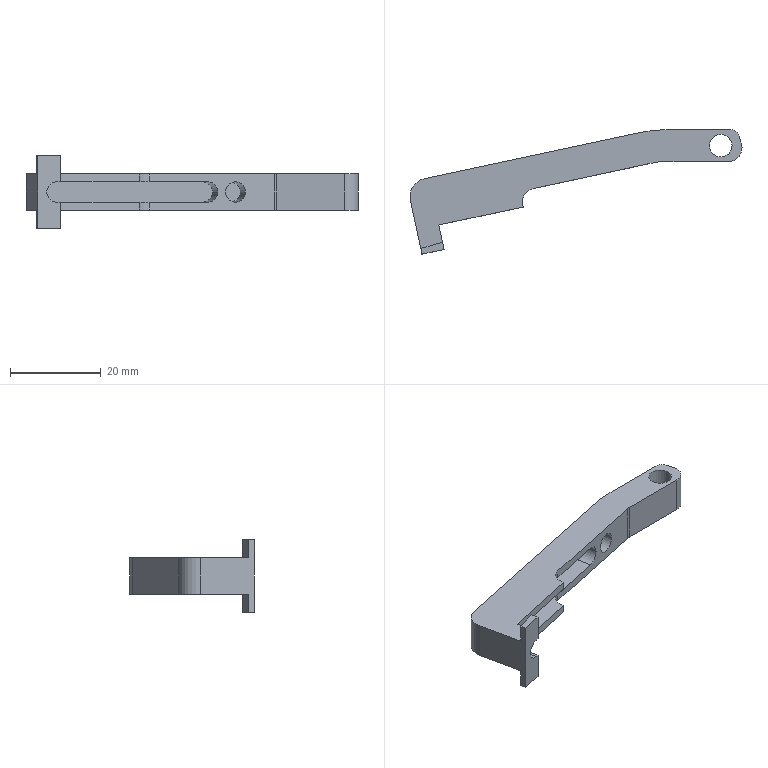Part | NX | features BREP 1 | 1 solid | 40 faces | box 73.222 x 27.429 x 16 mm | volume 3508 mm3 | plane 23 | cylinder 17 | commonest cylinder face diameters 6 x7 4.5 x5 5 x2 4 x1 8 x1 60 x1
STEP:
#1=CARTESIAN_POINT('',(-65.357,-7.291,4.));
#2=VERTEX_POINT('',#1);
#3=CARTESIAN_POINT('',(-68.43,-12.04,4.));
#4=VERTEX_POINT('',#3);
#5=CARTESIAN_POINT('',(-64.519,-11.202,4.));
#6=DIRECTION('',(0.,0.,1.));
#7=DIRECTION('',(1.,0.,0.));
#8=AXIS2_PLACEMENT_3D('',#5,#6,#7);
#9=CIRCLE('',#8,4.);
#10=EDGE_CURVE('',#2,#4,#9,.T.);
#11=ORIENTED_EDGE('',*,*,#10,.F.);
#12=CARTESIAN_POINT('',(-65.357,-7.291,-4.));
#13=VERTEX_POINT('',#12);
#14=CARTESIAN_POINT('',(-65.357,-7.291,4.));
#15=DIRECTION('',(0.,0.,1.));
#16=VECTOR('',#15,1000.);
#17=LINE('',#14,#16);
#18=EDGE_CURVE('',#13,#2,#17,.T.);
#19=ORIENTED_EDGE('',*,*,#18,.F.);
#20=CARTESIAN_POINT('',(-68.43,-12.04,-4.));
#21=VERTEX_POINT('',#20);
#22=CARTESIAN_POINT('',(-64.519,-11.202,-4.));
#23=DIRECTION('',(0.,0.,-1.));
#24=DIRECTION('',(1.,0.,0.));
#25=AXIS2_PLACEMENT_3D('',#22,#23,#24);
#26=CIRCLE('',#25,4.);
#27=EDGE_CURVE('',#21,#13,#26,.T.);
#28=ORIENTED_EDGE('',*,*,#27,.F.);
#29=CARTESIAN_POINT('',(-68.43,-12.04,-4.));
#30=DIRECTION('',(0.,0.,-1.));
#31=VECTOR('',#30,1000.);
#32=LINE('',#29,#31);
#33=EDGE_CURVE('',#4,#21,#32,.T.);
#34=ORIENTED_EDGE('',*,*,#33,.F.);
#35=EDGE_LOOP('',(#11,#19,#28,#34));
#36=FACE_BOUND('',#35,.T.);
#37=CARTESIAN_POINT('',(-64.519,-11.202,0.));
#38=DIRECTION('',(0.,0.,1.));
#39=DIRECTION('',(1.,0.,0.));
#40=AXIS2_PLACEMENT_3D('',#37,#38,#39);
#41=CYLINDRICAL_SURFACE('',#40,4.);
#42=ADVANCED_FACE('',(#36),#41,.T.);
#43=CARTESIAN_POINT('',(-66.144,-22.707,-8.));
#44=VERTEX_POINT('',#43);
#45=CARTESIAN_POINT('',(-61.334,-21.293,-8.));
#46=VERTEX_POINT('',#45);
#47=CARTESIAN_POINT('',(-56.523,-19.878,-8.));
#48=DIRECTION('',(0.9594,0.2821,0.));
#49=VECTOR('',#48,1000.);
#50=LINE('',#47,#49);
#51=EDGE_CURVE('',#44,#46,#50,.T.);
#52=ORIENTED_EDGE('',*,*,#51,.F.);
#53=CARTESIAN_POINT('',(-66.144,-22.707,-4.));
#54=VERTEX_POINT('',#53);
#55=CARTESIAN_POINT('',(-66.144,-22.707,0.));
#56=DIRECTION('',(0.,0.,-1.));
#57=VECTOR('',#56,1000.);
#58=LINE('',#55,#57);
#59=EDGE_CURVE('',#54,#44,#58,.T.);
#60=ORIENTED_EDGE('',*,*,#59,.F.);
#61=CARTESIAN_POINT('',(-61.334,-21.293,-4.));
#62=VERTEX_POINT('',#61);
#63=CARTESIAN_POINT('',(0.8821,-3.,-4.));
#64=DIRECTION('',(-0.9594,-0.2821,0.));
#65=VECTOR('',#64,1000.);
#66=LINE('',#63,#65);
#67=EDGE_CURVE('',#62,#54,#66,.T.);
#68=ORIENTED_EDGE('',*,*,#67,.F.);
#69=CARTESIAN_POINT('',(-61.334,-21.293,0.));
#70=DIRECTION('',(0.,0.,1.));
#71=VECTOR('',#70,1000.);
#72=LINE('',#69,#71);
#73=EDGE_CURVE('',#46,#62,#72,.T.);
#74=ORIENTED_EDGE('',*,*,#73,.F.);
#75=EDGE_LOOP('',(#52,#60,#68,#74));
#76=FACE_BOUND('',#75,.T.);
#77=CARTESIAN_POINT('',(-56.523,-19.878,0.));
#78=DIRECTION('',(0.2821,-0.9594,0.));
#79=DIRECTION('',(0.,0.,1.));
#80=AXIS2_PLACEMENT_3D('',#77,#78,#79);
#81=PLANE('',#80);
#82=ADVANCED_FACE('',(#76),#81,.F.);
#83=CARTESIAN_POINT('',(-66.144,-22.707,4.));
#84=VERTEX_POINT('',#83);
#85=CARTESIAN_POINT('',(-61.334,-21.293,4.));
#86=VERTEX_POINT('',#85);
#87=CARTESIAN_POINT('',(-56.523,-19.878,4.));
#88=DIRECTION('',(0.9594,0.2821,0.));
#89=VECTOR('',#88,1000.);
#90=LINE('',#87,#89);
#91=EDGE_CURVE('',#84,#86,#90,.T.);
#92=ORIENTED_EDGE('',*,*,#91,.F.);
#93=CARTESIAN_POINT('',(-66.144,-22.707,8.));
#94=VERTEX_POINT('',#93);
#95=CARTESIAN_POINT('',(-66.144,-22.707,0.));
#96=DIRECTION('',(0.,0.,-1.));
#97=VECTOR('',#96,1000.);
#98=LINE('',#95,#97);
#99=EDGE_CURVE('',#94,#84,#98,.T.);
#100=ORIENTED_EDGE('',*,*,#99,.F.);
#101=CARTESIAN_POINT('',(-61.334,-21.293,8.));
#102=VERTEX_POINT('',#101);
#103=CARTESIAN_POINT('',(-56.523,-19.878,8.));
#104=DIRECTION('',(-0.9594,-0.2821,0.));
#105=VECTOR('',#104,1000.);
#106=LINE('',#103,#105);
#107=EDGE_CURVE('',#102,#94,#106,.T.);
#108=ORIENTED_EDGE('',*,*,#107,.F.);
#109=CARTESIAN_POINT('',(-61.334,-21.293,0.));
#110=DIRECTION('',(0.,0.,1.));
#111=VECTOR('',#110,1000.);
#112=LINE('',#109,#111);
#113=EDGE_CURVE('',#86,#102,#112,.T.);
#114=ORIENTED_EDGE('',*,*,#113,.F.);
#115=EDGE_LOOP('',(#92,#100,#108,#114));
#116=FACE_BOUND('',#115,.T.);
#117=CARTESIAN_POINT('',(-56.523,-19.878,0.));
#118=DIRECTION('',(0.2821,-0.9594,0.));
#119=DIRECTION('',(0.,0.,1.));
#120=AXIS2_PLACEMENT_3D('',#117,#118,#119);
#121=PLANE('',#120);
#122=ADVANCED_FACE('',(#116),#121,.F.);
#123=CARTESIAN_POINT('',(-60.993,-22.881,2.25));
#124=VERTEX_POINT('',#123);
#125=CARTESIAN_POINT('',(-60.993,-22.881,8.));
#126=VERTEX_POINT('',#125);
#127=CARTESIAN_POINT('',(-60.993,-22.881,2.25));
#128=DIRECTION('',(0.,0.,1.));
#129=VECTOR('',#128,1000.);
#130=LINE('',#127,#129);
#131=EDGE_CURVE('',#124,#126,#130,.T.);
#132=ORIENTED_EDGE('',*,*,#131,.T.);
#133=CARTESIAN_POINT('',(-65.882,-23.929,8.));
#134=VERTEX_POINT('',#133);
#135=CARTESIAN_POINT('',(-65.882,-23.929,8.));
#136=DIRECTION('',(-0.9778,-0.2095,0.));
#137=VECTOR('',#136,1000.);
#138=LINE('',#135,#137);
#139=EDGE_CURVE('',#126,#134,#138,.T.);
#140=ORIENTED_EDGE('',*,*,#139,.T.);
#141=CARTESIAN_POINT('',(-65.882,-23.929,-8.));
#142=VERTEX_POINT('',#141);
#143=CARTESIAN_POINT('',(-65.882,-23.929,-8.));
#144=DIRECTION('',(0.,0.,-1.));
#145=VECTOR('',#144,1000.);
#146=LINE('',#143,#145);
#147=EDGE_CURVE('',#134,#142,#146,.T.);
#148=ORIENTED_EDGE('',*,*,#147,.T.);
#149=CARTESIAN_POINT('',(-60.993,-22.881,-8.));
#150=VERTEX_POINT('',#149);
#151=CARTESIAN_POINT('',(-65.882,-23.929,-8.));
#152=DIRECTION('',(0.9778,0.2095,0.));
#153=VECTOR('',#152,1000.);
#154=LINE('',#151,#153);
#155=EDGE_CURVE('',#142,#150,#154,.T.);
#156=ORIENTED_EDGE('',*,*,#155,.T.);
#157=CARTESIAN_POINT('',(-60.993,-22.881,-2.25));
#158=VERTEX_POINT('',#157);
#159=CARTESIAN_POINT('',(-60.993,-22.881,-8.));
#160=DIRECTION('',(0.,0.,1.));
#161=VECTOR('',#160,1000.);
#162=LINE('',#159,#161);
#163=EDGE_CURVE('',#150,#158,#162,.T.);
#164=ORIENTED_EDGE('',*,*,#163,.T.);
#165=CARTESIAN_POINT('',(-61.727,-23.039,-2.25));
#166=VERTEX_POINT('',#165);
#167=CARTESIAN_POINT('',(-61.727,-23.039,-2.25));
#168=DIRECTION('',(-0.9778,-0.2095,0.));
#169=VECTOR('',#168,1000.);
#170=LINE('',#167,#169);
#171=EDGE_CURVE('',#158,#166,#170,.T.);
#172=ORIENTED_EDGE('',*,*,#171,.T.);
#173=CARTESIAN_POINT('',(-61.727,-23.039,2.25));
#174=VERTEX_POINT('',#173);
#175=CARTESIAN_POINT('',(-61.727,-23.039,0.));
#176=DIRECTION('',(-0.2095,0.9778,0.));
#177=DIRECTION('',(0.9778,0.2095,0.));
#178=AXIS2_PLACEMENT_3D('',#175,#176,#177);
#179=CIRCLE('',#178,2.25);
#180=EDGE_CURVE('',#166,#174,#179,.T.);
#181=ORIENTED_EDGE('',*,*,#180,.T.);
#182=CARTESIAN_POINT('',(-60.993,-22.881,2.25));
#183=DIRECTION('',(0.9778,0.2095,0.));
#184=VECTOR('',#183,1000.);
#185=LINE('',#182,#184);
#186=EDGE_CURVE('',#174,#124,#185,.T.);
#187=ORIENTED_EDGE('',*,*,#186,.T.);
#188=EDGE_LOOP('',(#132,#140,#148,#156,#164,#172,#181,#187));
#189=FACE_BOUND('',#188,.T.);
#190=CARTESIAN_POINT('',(-61.727,-23.039,0.));
#191=DIRECTION('',(0.2095,-0.9778,0.));
#192=DIRECTION('',(0.9778,0.2095,0.));
#193=AXIS2_PLACEMENT_3D('',#190,#191,#192);
#194=PLANE('',#193);
#195=ADVANCED_FACE('',(#189),#194,.T.);
#196=ORIENTED_EDGE('',*,*,#73,.T.);
#197=CARTESIAN_POINT('',(-62.146,-17.504,-4.));
#198=VERTEX_POINT('',#197);
#199=CARTESIAN_POINT('',(-61.412,-20.926,-4.));
#200=DIRECTION('',(-0.2095,0.9778,0.));
#201=VECTOR('',#200,1000.);
#202=LINE('',#199,#201);
#203=EDGE_CURVE('',#62,#198,#202,.T.);
#204=ORIENTED_EDGE('',*,*,#203,.T.);
#205=CARTESIAN_POINT('',(-62.146,-17.504,-2.25));
#206=VERTEX_POINT('',#205);
#207=CARTESIAN_POINT('',(-62.146,-17.504,-8.));
#208=DIRECTION('',(0.,0.,1.));
#209=VECTOR('',#208,1000.);
#210=LINE('',#207,#209);
#211=EDGE_CURVE('',#198,#206,#210,.T.);
#212=ORIENTED_EDGE('',*,*,#211,.T.);
#213=CARTESIAN_POINT('',(-60.993,-22.881,-2.25));
#214=DIRECTION('',(-0.2095,0.9778,0.));
#215=VECTOR('',#214,1000.);
#216=LINE('',#213,#215);
#217=EDGE_CURVE('',#158,#206,#216,.T.);
#218=ORIENTED_EDGE('',*,*,#217,.F.);
#219=ORIENTED_EDGE('',*,*,#163,.F.);
#220=CARTESIAN_POINT('',(-60.993,-22.881,-8.));
#221=DIRECTION('',(-0.2095,0.9778,0.));
#222=VECTOR('',#221,1000.);
#223=LINE('',#220,#222);
#224=EDGE_CURVE('',#150,#46,#223,.T.);
#225=ORIENTED_EDGE('',*,*,#224,.T.);
#226=EDGE_LOOP('',(#196,#204,#212,#218,#219,#225));
#227=FACE_BOUND('',#226,.T.);
#228=CARTESIAN_POINT('',(-60.993,-22.881,-8.));
#229=DIRECTION('',(-0.9778,-0.2095,0.));
#230=DIRECTION('',(0.2095,-0.9778,0.));
#231=AXIS2_PLACEMENT_3D('',#228,#229,#230);
#232=PLANE('',#231);
#233=ADVANCED_FACE('',(#227),#232,.F.);
#234=CARTESIAN_POINT('',(-62.146,-17.504,4.));
#235=VERTEX_POINT('',#234);
#236=CARTESIAN_POINT('',(-61.412,-20.926,4.));
#237=DIRECTION('',(-0.2095,0.9778,0.));
#238=VECTOR('',#237,1000.);
#239=LINE('',#236,#238);
#240=EDGE_CURVE('',#86,#235,#239,.T.);
#241=ORIENTED_EDGE('',*,*,#240,.F.);
#242=ORIENTED_EDGE('',*,*,#113,.T.);
#243=CARTESIAN_POINT('',(-60.993,-22.881,8.));
#244=DIRECTION('',(-0.2095,0.9778,0.));
#245=VECTOR('',#244,1000.);
#246=LINE('',#243,#245);
#247=EDGE_CURVE('',#126,#102,#246,.T.);
#248=ORIENTED_EDGE('',*,*,#247,.F.);
#249=ORIENTED_EDGE('',*,*,#131,.F.);
#250=CARTESIAN_POINT('',(-62.146,-17.504,2.25));
#251=VERTEX_POINT('',#250);
#252=CARTESIAN_POINT('',(-60.993,-22.881,2.25));
#253=DIRECTION('',(-0.2095,0.9778,0.));
#254=VECTOR('',#253,1000.);
#255=LINE('',#252,#254);
#256=EDGE_CURVE('',#124,#251,#255,.T.);
#257=ORIENTED_EDGE('',*,*,#256,.T.);
#258=CARTESIAN_POINT('',(-62.146,-17.504,2.25));
#259=DIRECTION('',(0.,0.,1.));
#260=VECTOR('',#259,1000.);
#261=LINE('',#258,#260);
#262=EDGE_CURVE('',#251,#235,#261,.T.);
#263=ORIENTED_EDGE('',*,*,#262,.T.);
#264=EDGE_LOOP('',(#241,#242,#248,#249,#257,#263));
#265=FACE_BOUND('',#264,.T.);
#266=CARTESIAN_POINT('',(-60.993,-22.881,2.25));
#267=DIRECTION('',(-0.9778,-0.2095,0.));
#268=DIRECTION('',(0.2095,-0.9778,0.));
#269=AXIS2_PLACEMENT_3D('',#266,#267,#268);
#270=PLANE('',#269);
#271=ADVANCED_FACE('',(#265),#270,.F.);
#272=CARTESIAN_POINT('',(-64.765,-8.86,2.25));
#273=VERTEX_POINT('',#272);
#274=CARTESIAN_POINT('',(-73.303,30.984,2.25));
#275=DIRECTION('',(0.2095,-0.9778,0.));
#276=VECTOR('',#275,1000.);
#277=LINE('',#274,#276);
#278=EDGE_CURVE('',#273,#174,#277,.T.);
#279=ORIENTED_EDGE('',*,*,#278,.T.);
#280=ORIENTED_EDGE('',*,*,#180,.F.);
#281=CARTESIAN_POINT('',(-64.765,-8.86,-2.25));
#282=VERTEX_POINT('',#281);
#283=CARTESIAN_POINT('',(-73.303,30.984,-2.25));
#284=DIRECTION('',(0.2095,-0.9778,0.));
#285=VECTOR('',#284,1000.);
#286=LINE('',#283,#285);
#287=EDGE_CURVE('',#282,#166,#286,.T.);
#288=ORIENTED_EDGE('',*,*,#287,.F.);
#289=CARTESIAN_POINT('',(-64.765,-8.86,0.));
#290=DIRECTION('',(0.2095,-0.9778,0.));
#291=DIRECTION('',(-0.9778,-0.2095,0.));
#292=AXIS2_PLACEMENT_3D('',#289,#290,#291);
#293=CIRCLE('',#292,2.25);
#294=EDGE_CURVE('',#273,#282,#293,.T.);
#295=ORIENTED_EDGE('',*,*,#294,.F.);
#296=EDGE_LOOP('',(#279,#280,#288,#295));
#297=FACE_BOUND('',#296,.T.);
#298=CARTESIAN_POINT('',(-73.303,30.984,0.));
#299=DIRECTION('',(0.2095,-0.9778,0.));
#300=DIRECTION('',(0.9778,0.2095,0.));
#301=AXIS2_PLACEMENT_3D('',#298,#299,#300);
#302=CYLINDRICAL_SURFACE('',#301,2.25);
#303=ADVANCED_FACE('',(#297),#302,.F.);
#304=ORIENTED_EDGE('',*,*,#294,.T.);
#305=CARTESIAN_POINT('',(-29.564,-1.317,-2.25));
#306=VERTEX_POINT('',#305);
#307=CARTESIAN_POINT('',(-64.765,-8.86,-2.25));
#308=DIRECTION('',(0.9778,0.2095,0.));
#309=VECTOR('',#308,1000.);
#310=LINE('',#307,#309);
#311=EDGE_CURVE('',#282,#306,#310,.T.);
#312=ORIENTED_EDGE('',*,*,#311,.T.);
#313=CARTESIAN_POINT('',(-27.364,-0.846,0.));
#314=VERTEX_POINT('',#313);
#315=CARTESIAN_POINT('',(-29.564,-1.317,0.));
#316=DIRECTION('',(0.2095,-0.9778,0.));
#317=DIRECTION('',(-0.9778,-0.2095,0.));
#318=AXIS2_PLACEMENT_3D('',#315,#316,#317);
#319=CIRCLE('',#318,2.25);
#320=EDGE_CURVE('',#306,#314,#319,.T.);
#321=ORIENTED_EDGE('',*,*,#320,.T.);
#322=CARTESIAN_POINT('',(-29.564,-1.317,2.25));
#323=VERTEX_POINT('',#322);
#324=CARTESIAN_POINT('',(-29.564,-1.317,0.));
#325=DIRECTION('',(0.2095,-0.9778,0.));
#326=DIRECTION('',(-0.9778,-0.2095,0.));
#327=AXIS2_PLACEMENT_3D('',#324,#325,#326);
#328=CIRCLE('',#327,2.25);
#329=EDGE_CURVE('',#314,#323,#328,.T.);
#330=ORIENTED_EDGE('',*,*,#329,.T.);
#331=CARTESIAN_POINT('',(-64.765,-8.86,2.25));
#332=DIRECTION('',(-0.9778,-0.2095,0.));
#333=VECTOR('',#332,1000.);
#334=LINE('',#331,#333);
#335=EDGE_CURVE('',#323,#273,#334,.T.);
#336=ORIENTED_EDGE('',*,*,#335,.T.);
#337=EDGE_LOOP('',(#304,#312,#321,#330,#336));
#338=FACE_BOUND('',#337,.T.);
#339=CARTESIAN_POINT('',(-23.453,-0.007849,0.));
#340=DIRECTION('',(-0.2095,0.9778,0.));
#341=DIRECTION('',(-0.9778,-0.2095,0.));
#342=AXIS2_PLACEMENT_3D('',#339,#340,#341);
#343=PLANE('',#342);
#344=ADVANCED_FACE('',(#338),#343,.F.);
#345=CARTESIAN_POINT('',(-43.672,-13.034,2.25));
#346=VERTEX_POINT('',#345);
#347=CARTESIAN_POINT('',(-43.739,-12.405,2.25));
#348=VERTEX_POINT('',#347);
#349=CARTESIAN_POINT('',(-40.739,-12.405,2.25));
#350=DIRECTION('',(0.,0.,-1.));
#351=DIRECTION('',(1.,0.,0.));
#352=AXIS2_PLACEMENT_3D('',#349,#350,#351);
#353=CIRCLE('',#352,3.);
#354=EDGE_CURVE('',#346,#348,#353,.T.);
#355=ORIENTED_EDGE('',*,*,#354,.F.);
#356=CARTESIAN_POINT('',(-43.567,-13.522,2.25));
#357=VERTEX_POINT('',#356);
#358=CARTESIAN_POINT('',(-43.567,-13.522,2.25));
#359=DIRECTION('',(-0.2095,0.9778,0.));
#360=VECTOR('',#359,1000.);
#361=LINE('',#358,#360);
#362=EDGE_CURVE('',#357,#346,#361,.T.);
#363=ORIENTED_EDGE('',*,*,#362,.F.);
#364=CARTESIAN_POINT('',(-62.879,-17.661,2.25));
#365=DIRECTION('',(-0.9778,-0.2095,0.));
#366=VECTOR('',#365,1000.);
#367=LINE('',#364,#366);
#368=EDGE_CURVE('',#357,#251,#367,.T.);
#369=ORIENTED_EDGE('',*,*,#368,.T.);
#370=ORIENTED_EDGE('',*,*,#256,.F.);
#371=ORIENTED_EDGE('',*,*,#186,.F.);
#372=ORIENTED_EDGE('',*,*,#278,.F.);
#373=ORIENTED_EDGE('',*,*,#335,.F.);
#374=CARTESIAN_POINT('',(-28.411,-6.695,2.25));
#375=VERTEX_POINT('',#374);
#376=CARTESIAN_POINT('',(-38.102,38.527,2.25));
#377=DIRECTION('',(0.2095,-0.9778,0.));
#378=VECTOR('',#377,1000.);
#379=LINE('',#376,#378);
#380=EDGE_CURVE('',#323,#375,#379,.T.);
#381=ORIENTED_EDGE('',*,*,#380,.T.);
#382=CARTESIAN_POINT('',(-41.367,-9.472,2.25));
#383=VERTEX_POINT('',#382);
#384=CARTESIAN_POINT('',(-67.768,-15.129,2.25));
#385=DIRECTION('',(0.9778,0.2095,0.));
#386=VECTOR('',#385,1000.);
#387=LINE('',#384,#386);
#388=EDGE_CURVE('',#383,#375,#387,.T.);
#389=ORIENTED_EDGE('',*,*,#388,.F.);
#390=CARTESIAN_POINT('',(-40.739,-12.405,2.25));
#391=DIRECTION('',(0.,0.,-1.));
#392=DIRECTION('',(1.,0.,0.));
#393=AXIS2_PLACEMENT_3D('',#390,#391,#392);
#394=CIRCLE('',#393,3.);
#395=EDGE_CURVE('',#348,#383,#394,.T.);
#396=ORIENTED_EDGE('',*,*,#395,.F.);
#397=EDGE_LOOP('',(#355,#363,#369,#370,#371,#372,#373,#381,#389,#396));
#398=FACE_BOUND('',#397,.T.);
#399=CARTESIAN_POINT('',(-73.303,30.984,2.25));
#400=DIRECTION('',(0.,0.,1.));
#401=DIRECTION('',(1.,0.,0.));
#402=AXIS2_PLACEMENT_3D('',#399,#400,#401);
#403=PLANE('',#402);
#404=ADVANCED_FACE('',(#398),#403,.F.);
#405=CARTESIAN_POINT('',(-28.411,-6.695,-2.25));
#406=VERTEX_POINT('',#405);
#407=CARTESIAN_POINT('',(-38.102,38.527,-2.25));
#408=DIRECTION('',(0.2095,-0.9778,0.));
#409=VECTOR('',#408,1000.);
#410=LINE('',#407,#409);
#411=EDGE_CURVE('',#306,#406,#410,.T.);
#412=ORIENTED_EDGE('',*,*,#411,.F.);
#413=ORIENTED_EDGE('',*,*,#311,.F.);
#414=ORIENTED_EDGE('',*,*,#287,.T.);
#415=ORIENTED_EDGE('',*,*,#171,.F.);
#416=ORIENTED_EDGE('',*,*,#217,.T.);
#417=CARTESIAN_POINT('',(-43.567,-13.522,-2.25));
#418=VERTEX_POINT('',#417);
#419=CARTESIAN_POINT('',(-62.879,-17.661,-2.25));
#420=DIRECTION('',(0.9778,0.2095,0.));
#421=VECTOR('',#420,1000.);
#422=LINE('',#419,#421);
#423=EDGE_CURVE('',#206,#418,#422,.T.);
#424=ORIENTED_EDGE('',*,*,#423,.T.);
#425=CARTESIAN_POINT('',(-43.672,-13.034,-2.25));
#426=VERTEX_POINT('',#425);
#427=CARTESIAN_POINT('',(-43.567,-13.522,-2.25));
#428=DIRECTION('',(0.2095,-0.9778,0.));
#429=VECTOR('',#428,1000.);
#430=LINE('',#427,#429);
#431=EDGE_CURVE('',#426,#418,#430,.T.);
#432=ORIENTED_EDGE('',*,*,#431,.F.);
#433=CARTESIAN_POINT('',(-43.739,-12.405,-2.25));
#434=VERTEX_POINT('',#433);
#435=CARTESIAN_POINT('',(-40.739,-12.405,-2.25));
#436=DIRECTION('',(0.,0.,1.));
#437=DIRECTION('',(-1.,0.,0.));
#438=AXIS2_PLACEMENT_3D('',#435,#436,#437);
#439=CIRCLE('',#438,3.);
#440=EDGE_CURVE('',#434,#426,#439,.T.);
#441=ORIENTED_EDGE('',*,*,#440,.F.);
#442=CARTESIAN_POINT('',(-41.367,-9.472,-2.25));
#443=VERTEX_POINT('',#442);
#444=CARTESIAN_POINT('',(-40.739,-12.405,-2.25));
#445=DIRECTION('',(0.,0.,1.));
#446=DIRECTION('',(-1.,0.,0.));
#447=AXIS2_PLACEMENT_3D('',#444,#445,#446);
#448=CIRCLE('',#447,3.);
#449=EDGE_CURVE('',#443,#434,#448,.T.);
#450=ORIENTED_EDGE('',*,*,#449,.F.);
#451=CARTESIAN_POINT('',(-67.768,-15.129,-2.25));
#452=DIRECTION('',(-0.9778,-0.2095,0.));
#453=VECTOR('',#452,1000.);
#454=LINE('',#451,#453);
#455=EDGE_CURVE('',#406,#443,#454,.T.);
#456=ORIENTED_EDGE('',*,*,#455,.F.);
#457=EDGE_LOOP('',(#412,#413,#414,#415,#416,#424,#432,#441,#450,#456));
#458=FACE_BOUND('',#457,.T.);
#459=CARTESIAN_POINT('',(-73.303,30.984,-2.25));
#460=DIRECTION('',(0.,0.,-1.));
#461=DIRECTION('',(-1.,0.,0.));
#462=AXIS2_PLACEMENT_3D('',#459,#460,#461);
#463=PLANE('',#462);
#464=ADVANCED_FACE('',(#458),#463,.F.);
#465=CARTESIAN_POINT('',(-26.211,-6.224,0.));
#466=VERTEX_POINT('',#465);
#467=CARTESIAN_POINT('',(-35.902,38.999,0.));
#468=DIRECTION('',(0.2095,-0.9778,0.));
#469=VECTOR('',#468,1000.);
#470=LINE('',#467,#469);
#471=EDGE_CURVE('',#314,#466,#470,.T.);
#472=ORIENTED_EDGE('',*,*,#471,.F.);
#473=ORIENTED_EDGE('',*,*,#320,.F.);
#474=ORIENTED_EDGE('',*,*,#411,.T.);
#475=CARTESIAN_POINT('',(-28.411,-6.695,0.));
#476=DIRECTION('',(-0.2095,0.9778,0.));
#477=DIRECTION('',(-0.9778,-0.2095,0.));
#478=AXIS2_PLACEMENT_3D('',#475,#476,#477);
#479=CIRCLE('',#478,2.25);
#480=EDGE_CURVE('',#466,#406,#479,.T.);
#481=ORIENTED_EDGE('',*,*,#480,.F.);
#482=EDGE_LOOP('',(#472,#473,#474,#481));
#483=FACE_BOUND('',#482,.T.);
#484=CARTESIAN_POINT('',(-38.102,38.527,0.));
#485=DIRECTION('',(0.2095,-0.9778,0.));
#486=DIRECTION('',(0.9778,0.2095,0.));
#487=AXIS2_PLACEMENT_3D('',#484,#485,#486);
#488=CYLINDRICAL_SURFACE('',#487,2.25);
#489=ADVANCED_FACE('',(#483),#488,.F.);
#490=CARTESIAN_POINT('',(4.703,-0.5,-4.));
#491=VERTEX_POINT('',#490);
#492=CARTESIAN_POINT('',(4.703,-0.5,4.));
#493=VERTEX_POINT('',#492);
#494=CARTESIAN_POINT('',(4.703,-0.5,4.));
#495=DIRECTION('',(0.,0.,1.));
#496=VECTOR('',#495,1000.);
#497=LINE('',#494,#496);
#498=EDGE_CURVE('',#491,#493,#497,.T.);
#499=ORIENTED_EDGE('',*,*,#498,.F.);
#500=CARTESIAN_POINT('',(4.587,0.3242,-4.));
#501=VERTEX_POINT('',#500);
#502=CARTESIAN_POINT('',(1.703,-0.5,-4.));
#503=DIRECTION('',(0.,0.,-1.));
#504=DIRECTION('',(1.,0.,0.));
#505=AXIS2_PLACEMENT_3D('',#502,#503,#504);
#506=CIRCLE('',#505,3.);
#507=EDGE_CURVE('',#501,#491,#506,.T.);
#508=ORIENTED_EDGE('',*,*,#507,.F.);
#509=CARTESIAN_POINT('',(4.587,0.3242,4.));
#510=VERTEX_POINT('',#509);
#511=CARTESIAN_POINT('',(4.587,0.3242,-4.));
#512=DIRECTION('',(0.,0.,-1.));
#513=VECTOR('',#512,1000.);
#514=LINE('',#511,#513);
#515=EDGE_CURVE('',#510,#501,#514,.T.);
#516=ORIENTED_EDGE('',*,*,#515,.F.);
#517=CARTESIAN_POINT('',(1.703,-0.5,4.));
#518=DIRECTION('',(0.,0.,1.));
#519=DIRECTION('',(1.,0.,0.));
#520=AXIS2_PLACEMENT_3D('',#517,#518,#519);
#521=CIRCLE('',#520,3.);
#522=EDGE_CURVE('',#493,#510,#521,.T.);
#523=ORIENTED_EDGE('',*,*,#522,.F.);
#524=EDGE_LOOP('',(#499,#508,#516,#523));
#525=FACE_BOUND('',#524,.T.);
#526=CARTESIAN_POINT('',(1.703,-0.5,4.));
#527=DIRECTION('',(0.,0.,1.));
#528=DIRECTION('',(1.,0.,0.));
#529=AXIS2_PLACEMENT_3D('',#526,#527,#528);
#530=CYLINDRICAL_SURFACE('',#529,3.);
#531=ADVANCED_FACE('',(#525),#530,.T.);
#532=CARTESIAN_POINT('',(2.171,3.5,-4.));
#533=VERTEX_POINT('',#532);
#534=CARTESIAN_POINT('',(4.095,2.049,-4.));
#535=VERTEX_POINT('',#534);
#536=CARTESIAN_POINT('',(2.171,1.5,-4.));
#537=DIRECTION('',(0.,0.,-1.));
#538=DIRECTION('',(1.,0.,0.));
#539=AXIS2_PLACEMENT_3D('',#536,#537,#538);
#540=CIRCLE('',#539,2.);
#541=EDGE_CURVE('',#533,#535,#540,.T.);
#542=ORIENTED_EDGE('',*,*,#541,.F.);
#543=CARTESIAN_POINT('',(2.171,3.5,4.));
#544=VERTEX_POINT('',#543);
#545=CARTESIAN_POINT('',(2.171,3.5,-4.));
#546=DIRECTION('',(0.,0.,-1.));
#547=VECTOR('',#546,1000.);
#548=LINE('',#545,#547);
#549=EDGE_CURVE('',#544,#533,#548,.T.);
#550=ORIENTED_EDGE('',*,*,#549,.F.);
#551=CARTESIAN_POINT('',(4.095,2.049,4.));
#552=VERTEX_POINT('',#551);
#553=CARTESIAN_POINT('',(2.171,1.5,4.));
#554=DIRECTION('',(0.,0.,1.));
#555=DIRECTION('',(1.,0.,0.));
#556=AXIS2_PLACEMENT_3D('',#553,#554,#555);
#557=CIRCLE('',#556,2.);
#558=EDGE_CURVE('',#552,#544,#557,.T.);
#559=ORIENTED_EDGE('',*,*,#558,.F.);
#560=CARTESIAN_POINT('',(4.095,2.049,4.));
#561=DIRECTION('',(0.,0.,1.));
#562=VECTOR('',#561,1000.);
#563=LINE('',#560,#562);
#564=EDGE_CURVE('',#535,#552,#563,.T.);
#565=ORIENTED_EDGE('',*,*,#564,.F.);
#566=EDGE_LOOP('',(#542,#550,#559,#565));
#567=FACE_BOUND('',#566,.T.);
#568=CARTESIAN_POINT('',(2.171,1.5,-4.));
#569=DIRECTION('',(0.,0.,-1.));
#570=DIRECTION('',(-1.,0.,0.));
#571=AXIS2_PLACEMENT_3D('',#568,#569,#570);
#572=CYLINDRICAL_SURFACE('',#571,2.);
#573=ADVANCED_FACE('',(#567),#572,.T.);
#574=CARTESIAN_POINT('',(3.68,3.5,-4.));
#575=DIRECTION('',(0.2747,-0.9615,0.));
#576=VECTOR('',#575,1000.);
#577=LINE('',#574,#576);
#578=EDGE_CURVE('',#535,#501,#577,.T.);
#579=ORIENTED_EDGE('',*,*,#578,.F.);
#580=ORIENTED_EDGE('',*,*,#564,.T.);
#581=CARTESIAN_POINT('',(3.68,3.5,4.));
#582=DIRECTION('',(0.2747,-0.9615,0.));
#583=VECTOR('',#582,1000.);
#584=LINE('',#581,#583);
#585=EDGE_CURVE('',#552,#510,#584,.T.);
#586=ORIENTED_EDGE('',*,*,#585,.T.);
#587=ORIENTED_EDGE('',*,*,#515,.T.);
#588=EDGE_LOOP('',(#579,#580,#586,#587));
#589=FACE_BOUND('',#588,.T.);
#590=CARTESIAN_POINT('',(3.68,3.5,-4.));
#591=DIRECTION('',(-0.9615,-0.2747,0.));
#592=DIRECTION('',(0.2747,-0.9615,0.));
#593=AXIS2_PLACEMENT_3D('',#590,#591,#592);
#594=PLANE('',#593);
#595=ADVANCED_FACE('',(#589),#594,.F.);
#596=CARTESIAN_POINT('',(-13.811,-3.567,4.));
#597=VERTEX_POINT('',#596);
#598=CARTESIAN_POINT('',(-13.182,-3.5,4.));
#599=VERTEX_POINT('',#598);
#600=CARTESIAN_POINT('',(-13.182,-6.5,4.));
#601=DIRECTION('',(0.,0.,-1.));
#602=DIRECTION('',(1.,0.,0.));
#603=AXIS2_PLACEMENT_3D('',#600,#601,#602);
#604=CIRCLE('',#603,3.);
#605=EDGE_CURVE('',#597,#599,#604,.T.);
#606=ORIENTED_EDGE('',*,*,#605,.F.);
#607=CARTESIAN_POINT('',(-13.811,-3.567,-4.));
#608=VERTEX_POINT('',#607);
#609=CARTESIAN_POINT('',(-13.811,-3.567,4.));
#610=DIRECTION('',(0.,0.,1.));
#611=VECTOR('',#610,1000.);
#612=LINE('',#609,#611);
#613=EDGE_CURVE('',#608,#597,#612,.T.);
#614=ORIENTED_EDGE('',*,*,#613,.F.);
#615=CARTESIAN_POINT('',(-13.182,-3.5,-4.));
#616=VERTEX_POINT('',#615);
#617=CARTESIAN_POINT('',(-13.182,-6.5,-4.));
#618=DIRECTION('',(0.,0.,1.));
#619=DIRECTION('',(1.,0.,0.));
#620=AXIS2_PLACEMENT_3D('',#617,#618,#619);
#621=CIRCLE('',#620,3.);
#622=EDGE_CURVE('',#616,#608,#621,.T.);
#623=ORIENTED_EDGE('',*,*,#622,.F.);
#624=CARTESIAN_POINT('',(-13.182,-3.5,-4.));
#625=DIRECTION('',(0.,0.,-1.));
#626=VECTOR('',#625,1000.);
#627=LINE('',#624,#626);
#628=EDGE_CURVE('',#599,#616,#627,.T.);
#629=ORIENTED_EDGE('',*,*,#628,.F.);
#630=EDGE_LOOP('',(#606,#614,#623,#629));
#631=FACE_BOUND('',#630,.T.);
#632=CARTESIAN_POINT('',(-13.182,-6.5,4.));
#633=DIRECTION('',(0.,0.,1.));
#634=DIRECTION('',(1.,0.,0.));
#635=AXIS2_PLACEMENT_3D('',#632,#633,#634);
#636=CYLINDRICAL_SURFACE('',#635,3.);
#637=ADVANCED_FACE('',(#631),#636,.F.);
#638=CARTESIAN_POINT('',(-43.739,-12.405,4.));
#639=VERTEX_POINT('',#638);
#640=CARTESIAN_POINT('',(-43.739,-12.405,4.));
#641=DIRECTION('',(0.,0.,-1.));
#642=VECTOR('',#641,1000.);
#643=LINE('',#640,#642);
#644=EDGE_CURVE('',#639,#348,#643,.T.);
#645=ORIENTED_EDGE('',*,*,#644,.F.);
#646=CARTESIAN_POINT('',(-43.672,-13.034,4.));
#647=VERTEX_POINT('',#646);
#648=CARTESIAN_POINT('',(-40.739,-12.405,4.));
#649=DIRECTION('',(0.,0.,-1.));
#650=DIRECTION('',(1.,0.,0.));
#651=AXIS2_PLACEMENT_3D('',#648,#649,#650);
#652=CIRCLE('',#651,3.);
#653=EDGE_CURVE('',#647,#639,#652,.T.);
#654=ORIENTED_EDGE('',*,*,#653,.F.);
#655=CARTESIAN_POINT('',(-43.672,-13.034,4.));
#656=DIRECTION('',(0.,0.,1.));
#657=VECTOR('',#656,1000.);
#658=LINE('',#655,#657);
#659=EDGE_CURVE('',#346,#647,#658,.T.);
#660=ORIENTED_EDGE('',*,*,#659,.F.);
#661=ORIENTED_EDGE('',*,*,#354,.T.);
#662=EDGE_LOOP('',(#645,#654,#660,#661));
#663=FACE_BOUND('',#662,.T.);
#664=CARTESIAN_POINT('',(-40.739,-12.405,4.));
#665=DIRECTION('',(0.,0.,-1.));
#666=DIRECTION('',(-1.,0.,0.));
#667=AXIS2_PLACEMENT_3D('',#664,#665,#666);
#668=CYLINDRICAL_SURFACE('',#667,3.);
#669=ADVANCED_FACE('',(#663),#668,.F.);
#670=CARTESIAN_POINT('',(-21.253,0.4636,0.));
#671=VERTEX_POINT('',#670);
#672=CARTESIAN_POINT('',(-25.653,-0.4793,0.));
#673=VERTEX_POINT('',#672);
#674=CARTESIAN_POINT('',(-23.453,-0.007849,0.));
#675=DIRECTION('',(-0.2095,0.9778,0.));
#676=DIRECTION('',(-0.9778,-0.2095,0.));
#677=AXIS2_PLACEMENT_3D('',#674,#675,#676);
#678=CIRCLE('',#677,2.25);
#679=EDGE_CURVE('',#671,#673,#678,.T.);
#680=ORIENTED_EDGE('',*,*,#679,.F.);
#681=CARTESIAN_POINT('',(-23.453,-0.007849,0.));
#682=DIRECTION('',(-0.2095,0.9778,0.));
#683=DIRECTION('',(-0.9778,-0.2095,0.));
#684=AXIS2_PLACEMENT_3D('',#681,#682,#683);
#685=CIRCLE('',#684,2.25);
#686=EDGE_CURVE('',#673,#671,#685,.T.);
#687=ORIENTED_EDGE('',*,*,#686,.F.);
#688=EDGE_LOOP('',(#680,#687));
#689=FACE_BOUND('',#688,.T.);
#690=CARTESIAN_POINT('',(-23.453,-0.007849,0.));
#691=DIRECTION('',(-0.2095,0.9778,0.));
#692=DIRECTION('',(-0.9778,-0.2095,0.));
#693=AXIS2_PLACEMENT_3D('',#690,#691,#692);
#694=PLANE('',#693);
#695=ADVANCED_FACE('',(#689),#694,.F.);
#696=CARTESIAN_POINT('',(-24.5,-5.857,0.));
#697=VERTEX_POINT('',#696);
#698=CARTESIAN_POINT('',(-25.653,-0.4793,0.));
#699=DIRECTION('',(0.2095,-0.9778,0.));
#700=VECTOR('',#699,1000.);
#701=LINE('',#698,#700);
#702=EDGE_CURVE('',#697,#673,#701,.F.);
#703=ORIENTED_EDGE('',*,*,#702,.T.);
#704=ORIENTED_EDGE('',*,*,#686,.T.);
#705=CARTESIAN_POINT('',(-20.1,-4.914,0.));
#706=VERTEX_POINT('',#705);
#707=CARTESIAN_POINT('',(-21.253,0.4636,0.));
#708=DIRECTION('',(0.2095,-0.9778,0.));
#709=VECTOR('',#708,1000.);
#710=LINE('',#707,#709);
#711=EDGE_CURVE('',#706,#671,#710,.F.);
#712=ORIENTED_EDGE('',*,*,#711,.F.);
#713=CARTESIAN_POINT('',(-22.3,-5.386,0.));
#714=DIRECTION('',(0.2095,-0.9778,0.));
#715=DIRECTION('',(-0.9778,-0.2095,0.));
#716=AXIS2_PLACEMENT_3D('',#713,#714,#715);
#717=CIRCLE('',#716,2.25);
#718=EDGE_CURVE('',#706,#697,#717,.T.);
#719=ORIENTED_EDGE('',*,*,#718,.T.);
#720=EDGE_LOOP('',(#703,#704,#712,#719));
#721=FACE_BOUND('',#720,.T.);
#722=CARTESIAN_POINT('',(-23.453,-0.007849,0.));
#723=DIRECTION('',(0.2095,-0.9778,0.));
#724=DIRECTION('',(0.9778,0.2095,0.));
#725=AXIS2_PLACEMENT_3D('',#722,#723,#724);
#726=CYLINDRICAL_SURFACE('',#725,2.25);
#727=ADVANCED_FACE('',(#721),#726,.F.);
#728=CARTESIAN_POINT('',(-11.822,3.5,4.));
#729=VERTEX_POINT('',#728);
#730=CARTESIAN_POINT('',(-18.108,2.834,4.));
#731=VERTEX_POINT('',#730);
#732=CARTESIAN_POINT('',(-11.822,-26.5,4.));
#733=DIRECTION('',(0.,0.,1.));
#734=DIRECTION('',(1.,0.,0.));
#735=AXIS2_PLACEMENT_3D('',#732,#733,#734);
#736=CIRCLE('',#735,30.);
#737=EDGE_CURVE('',#729,#731,#736,.T.);
#738=ORIENTED_EDGE('',*,*,#737,.F.);
#739=CARTESIAN_POINT('',(-11.822,3.5,-4.));
#740=VERTEX_POINT('',#739);
#741=CARTESIAN_POINT('',(-11.822,3.5,4.));
#742=DIRECTION('',(0.,0.,1.));
#743=VECTOR('',#742,1000.);
#744=LINE('',#741,#743);
#745=EDGE_CURVE('',#740,#729,#744,.T.);
#746=ORIENTED_EDGE('',*,*,#745,.F.);
#747=CARTESIAN_POINT('',(-18.108,2.834,-4.));
#748=VERTEX_POINT('',#747);
#749=CARTESIAN_POINT('',(-11.822,-26.5,-4.));
#750=DIRECTION('',(0.,0.,-1.));
#751=DIRECTION('',(1.,0.,0.));
#752=AXIS2_PLACEMENT_3D('',#749,#750,#751);
#753=CIRCLE('',#752,30.);
#754=EDGE_CURVE('',#748,#740,#753,.T.);
#755=ORIENTED_EDGE('',*,*,#754,.F.);
#756=CARTESIAN_POINT('',(-18.108,2.834,-4.));
#757=DIRECTION('',(0.,0.,-1.));
#758=VECTOR('',#757,1000.);
#759=LINE('',#756,#758);
#760=EDGE_CURVE('',#731,#748,#759,.T.);
#761=ORIENTED_EDGE('',*,*,#760,.F.);
#762=EDGE_LOOP('',(#738,#746,#755,#761));
#763=FACE_BOUND('',#762,.T.);
#764=CARTESIAN_POINT('',(-11.822,-26.5,4.));
#765=DIRECTION('',(0.,0.,1.));
#766=DIRECTION('',(1.,0.,0.));
#767=AXIS2_PLACEMENT_3D('',#764,#765,#766);
#768=CYLINDRICAL_SURFACE('',#767,30.);
#769=ADVANCED_FACE('',(#763),#768,.T.);
#770=CARTESIAN_POINT('',(-43.567,-13.522,4.));
#771=VERTEX_POINT('',#770);
#772=CARTESIAN_POINT('',(-43.567,-13.522,4.));
#773=DIRECTION('',(0.,0.,1.));
#774=VECTOR('',#773,1000.);
#775=LINE('',#772,#774);
#776=EDGE_CURVE('',#357,#771,#775,.T.);
#777=ORIENTED_EDGE('',*,*,#776,.F.);
#778=ORIENTED_EDGE('',*,*,#362,.T.);
#779=ORIENTED_EDGE('',*,*,#659,.T.);
#780=CARTESIAN_POINT('',(-43.567,-13.522,4.));
#781=DIRECTION('',(-0.2095,0.9778,0.));
#782=VECTOR('',#781,1000.);
#783=LINE('',#780,#782);
#784=EDGE_CURVE('',#771,#647,#783,.T.);
#785=ORIENTED_EDGE('',*,*,#784,.F.);
#786=EDGE_LOOP('',(#777,#778,#779,#785));
#787=FACE_BOUND('',#786,.T.);
#788=CARTESIAN_POINT('',(-43.567,-13.522,4.));
#789=DIRECTION('',(-0.9778,-0.2095,0.));
#790=DIRECTION('',(0.2095,-0.9778,0.));
#791=AXIS2_PLACEMENT_3D('',#788,#789,#790);
#792=PLANE('',#791);
#793=ADVANCED_FACE('',(#787),#792,.F.);
#794=CARTESIAN_POINT('',(-67.768,-15.129,4.));
#795=DIRECTION('',(-0.2095,0.9778,0.));
#796=VECTOR('',#795,1000.);
#797=LINE('',#794,#796);
#798=EDGE_CURVE('',#84,#4,#797,.T.);
#799=ORIENTED_EDGE('',*,*,#798,.T.);
#800=ORIENTED_EDGE('',*,*,#33,.T.);
#801=CARTESIAN_POINT('',(-69.268,-8.129,-4.));
#802=DIRECTION('',(0.2095,-0.9778,0.));
#803=VECTOR('',#802,1000.);
#804=LINE('',#801,#803);
#805=EDGE_CURVE('',#21,#54,#804,.T.);
#806=ORIENTED_EDGE('',*,*,#805,.T.);
#807=ORIENTED_EDGE('',*,*,#59,.T.);
#808=CARTESIAN_POINT('',(-65.882,-23.929,-8.));
#809=DIRECTION('',(-0.2095,0.9778,0.));
#810=VECTOR('',#809,1000.);
#811=LINE('',#808,#810);
#812=EDGE_CURVE('',#142,#44,#811,.T.);
#813=ORIENTED_EDGE('',*,*,#812,.F.);
#814=ORIENTED_EDGE('',*,*,#147,.F.);
#815=CARTESIAN_POINT('',(-65.882,-23.929,8.));
#816=DIRECTION('',(-0.2095,0.9778,0.));
#817=VECTOR('',#816,1000.);
#818=LINE('',#815,#817);
#819=EDGE_CURVE('',#134,#94,#818,.T.);
#820=ORIENTED_EDGE('',*,*,#819,.T.);
#821=ORIENTED_EDGE('',*,*,#99,.T.);
#822=EDGE_LOOP('',(#799,#800,#806,#807,#813,#814,#820,#821));
#823=FACE_BOUND('',#822,.T.);
#824=CARTESIAN_POINT('',(-67.892,-14.548,0.));
#825=DIRECTION('',(-0.9778,-0.2095,0.));
#826=DIRECTION('',(0.2095,-0.9778,0.));
#827=AXIS2_PLACEMENT_3D('',#824,#825,#826);
#828=PLANE('',#827);
#829=ADVANCED_FACE('',(#823),#828,.T.);
#830=CARTESIAN_POINT('',(-69.268,-8.129,-4.));
#831=DIRECTION('',(0.9778,0.2095,0.));
#832=VECTOR('',#831,1000.);
#833=LINE('',#830,#832);
#834=EDGE_CURVE('',#13,#748,#833,.T.);
#835=ORIENTED_EDGE('',*,*,#834,.F.);
#836=ORIENTED_EDGE('',*,*,#18,.T.);
#837=CARTESIAN_POINT('',(-69.268,-8.129,4.));
#838=DIRECTION('',(0.9778,0.2095,0.));
#839=VECTOR('',#838,1000.);
#840=LINE('',#837,#839);
#841=EDGE_CURVE('',#2,#731,#840,.T.);
#842=ORIENTED_EDGE('',*,*,#841,.T.);
#843=ORIENTED_EDGE('',*,*,#760,.T.);
#844=EDGE_LOOP('',(#835,#836,#842,#843));
#845=FACE_BOUND('',#844,.T.);
#846=CARTESIAN_POINT('',(-69.268,-8.129,4.));
#847=DIRECTION('',(0.2095,-0.9778,0.));
#848=DIRECTION('',(0.9778,0.2095,0.));
#849=AXIS2_PLACEMENT_3D('',#846,#847,#848);
#850=PLANE('',#849);
#851=ADVANCED_FACE('',(#845),#850,.F.);
#852=ORIENTED_EDGE('',*,*,#805,.F.);
#853=ORIENTED_EDGE('',*,*,#27,.T.);
#854=ORIENTED_EDGE('',*,*,#834,.T.);
#855=ORIENTED_EDGE('',*,*,#754,.T.);
#856=CARTESIAN_POINT('',(0.,3.5,-4.));
#857=DIRECTION('',(1.,0.,0.));
#858=VECTOR('',#857,1000.);
#859=LINE('',#856,#858);
#860=EDGE_CURVE('',#740,#533,#859,.T.);
#861=ORIENTED_EDGE('',*,*,#860,.T.);
#862=ORIENTED_EDGE('',*,*,#541,.T.);
#863=ORIENTED_EDGE('',*,*,#578,.T.);
#864=ORIENTED_EDGE('',*,*,#507,.T.);
#865=CARTESIAN_POINT('',(1.703,-3.5,-4.));
#866=VERTEX_POINT('',#865);
#867=CARTESIAN_POINT('',(1.703,-0.5,-4.));
#868=DIRECTION('',(0.,0.,-1.));
#869=DIRECTION('',(1.,0.,0.));
#870=AXIS2_PLACEMENT_3D('',#867,#868,#869);
#871=CIRCLE('',#870,3.);
#872=EDGE_CURVE('',#491,#866,#871,.T.);
#873=ORIENTED_EDGE('',*,*,#872,.T.);
#874=CARTESIAN_POINT('',(0.,-3.5,-4.));
#875=DIRECTION('',(1.,0.,0.));
#876=VECTOR('',#875,1000.);
#877=LINE('',#874,#876);
#878=EDGE_CURVE('',#616,#866,#877,.T.);
#879=ORIENTED_EDGE('',*,*,#878,.F.);
#880=ORIENTED_EDGE('',*,*,#622,.T.);
#881=CARTESIAN_POINT('',(-41.367,-9.472,-4.));
#882=VERTEX_POINT('',#881);
#883=CARTESIAN_POINT('',(-67.768,-15.129,-4.));
#884=DIRECTION('',(0.9778,0.2095,0.));
#885=VECTOR('',#884,1000.);
#886=LINE('',#883,#885);
#887=EDGE_CURVE('',#882,#608,#886,.T.);
#888=ORIENTED_EDGE('',*,*,#887,.F.);
#889=CARTESIAN_POINT('',(-43.739,-12.405,-4.));
#890=VERTEX_POINT('',#889);
#891=CARTESIAN_POINT('',(-40.739,-12.405,-4.));
#892=DIRECTION('',(0.,0.,1.));
#893=DIRECTION('',(1.,0.,0.));
#894=AXIS2_PLACEMENT_3D('',#891,#892,#893);
#895=CIRCLE('',#894,3.);
#896=EDGE_CURVE('',#882,#890,#895,.T.);
#897=ORIENTED_EDGE('',*,*,#896,.T.);
#898=CARTESIAN_POINT('',(-43.672,-13.034,-4.));
#899=VERTEX_POINT('',#898);
#900=CARTESIAN_POINT('',(-40.739,-12.405,-4.));
#901=DIRECTION('',(0.,0.,1.));
#902=DIRECTION('',(1.,0.,0.));
#903=AXIS2_PLACEMENT_3D('',#900,#901,#902);
#904=CIRCLE('',#903,3.);
#905=EDGE_CURVE('',#890,#899,#904,.T.);
#906=ORIENTED_EDGE('',*,*,#905,.T.);
#907=CARTESIAN_POINT('',(-43.567,-13.522,-4.));
#908=VERTEX_POINT('',#907);
#909=CARTESIAN_POINT('',(-43.567,-13.522,-4.));
#910=DIRECTION('',(-0.2095,0.9778,0.));
#911=VECTOR('',#910,1000.);
#912=LINE('',#909,#911);
#913=EDGE_CURVE('',#908,#899,#912,.T.);
#914=ORIENTED_EDGE('',*,*,#913,.F.);
#915=CARTESIAN_POINT('',(-67.035,-18.551,-4.));
#916=DIRECTION('',(0.9778,0.2095,0.));
#917=VECTOR('',#916,1000.);
#918=LINE('',#915,#917);
#919=EDGE_CURVE('',#198,#908,#918,.T.);
#920=ORIENTED_EDGE('',*,*,#919,.F.);
#921=ORIENTED_EDGE('',*,*,#203,.F.);
#922=ORIENTED_EDGE('',*,*,#67,.T.);
#923=EDGE_LOOP('',(#852,#853,#854,#855,#861,#862,#863,#864,#873,#879,#880,#888,#897,#906,#914,#920,#921,#922));
#924=FACE_BOUND('',#923,.T.);
#925=CARTESIAN_POINT('',(-2.5,0.,-4.));
#926=VERTEX_POINT('',#925);
#927=CARTESIAN_POINT('',(2.5,0.,-4.));
#928=VERTEX_POINT('',#927);
#929=CARTESIAN_POINT('',(0.,0.,-4.));
#930=DIRECTION('',(0.,0.,1.));
#931=DIRECTION('',(1.,0.,0.));
#932=AXIS2_PLACEMENT_3D('',#929,#930,#931);
#933=CIRCLE('',#932,2.5);
#934=EDGE_CURVE('',#926,#928,#933,.T.);
#935=ORIENTED_EDGE('',*,*,#934,.T.);
#936=CARTESIAN_POINT('',(0.,0.,-4.));
#937=DIRECTION('',(0.,0.,1.));
#938=DIRECTION('',(1.,0.,0.));
#939=AXIS2_PLACEMENT_3D('',#936,#937,#938);
#940=CIRCLE('',#939,2.5);
#941=EDGE_CURVE('',#928,#926,#940,.T.);
#942=ORIENTED_EDGE('',*,*,#941,.T.);
#943=EDGE_LOOP('',(#935,#942));
#944=FACE_BOUND('',#943,.T.);
#945=CARTESIAN_POINT('',(0.,0.,-4.));
#946=DIRECTION('',(0.,0.,1.));
#947=DIRECTION('',(1.,0.,0.));
#948=AXIS2_PLACEMENT_3D('',#945,#946,#947);
#949=PLANE('',#948);
#950=ADVANCED_FACE('',(#924,#944),#949,.F.);
#951=CARTESIAN_POINT('',(-2.5,0.,4.));
#952=VERTEX_POINT('',#951);
#953=CARTESIAN_POINT('',(2.5,0.,4.));
#954=VERTEX_POINT('',#953);
#955=CARTESIAN_POINT('',(0.,0.,4.));
#956=DIRECTION('',(0.,0.,1.));
#957=DIRECTION('',(1.,0.,0.));
#958=AXIS2_PLACEMENT_3D('',#955,#956,#957);
#959=CIRCLE('',#958,2.5);
#960=EDGE_CURVE('',#952,#954,#959,.T.);
#961=ORIENTED_EDGE('',*,*,#960,.F.);
#962=CARTESIAN_POINT('',(0.,0.,4.));
#963=DIRECTION('',(0.,0.,1.));
#964=DIRECTION('',(1.,0.,0.));
#965=AXIS2_PLACEMENT_3D('',#962,#963,#964);
#966=CIRCLE('',#965,2.5);
#967=EDGE_CURVE('',#954,#952,#966,.T.);
#968=ORIENTED_EDGE('',*,*,#967,.F.);
#969=EDGE_LOOP('',(#961,#968));
#970=FACE_BOUND('',#969,.T.);
#971=ORIENTED_EDGE('',*,*,#841,.F.);
#972=ORIENTED_EDGE('',*,*,#10,.T.);
#973=ORIENTED_EDGE('',*,*,#798,.F.);
#974=ORIENTED_EDGE('',*,*,#91,.T.);
#975=ORIENTED_EDGE('',*,*,#240,.T.);
#976=CARTESIAN_POINT('',(-67.035,-18.551,4.));
#977=DIRECTION('',(-0.9778,-0.2095,0.));
#978=VECTOR('',#977,1000.);
#979=LINE('',#976,#978);
#980=EDGE_CURVE('',#771,#235,#979,.T.);
#981=ORIENTED_EDGE('',*,*,#980,.F.);
#982=ORIENTED_EDGE('',*,*,#784,.T.);
#983=ORIENTED_EDGE('',*,*,#653,.T.);
#984=CARTESIAN_POINT('',(-41.367,-9.472,4.));
#985=VERTEX_POINT('',#984);
#986=CARTESIAN_POINT('',(-40.739,-12.405,4.));
#987=DIRECTION('',(0.,0.,-1.));
#988=DIRECTION('',(1.,0.,0.));
#989=AXIS2_PLACEMENT_3D('',#986,#987,#988);
#990=CIRCLE('',#989,3.);
#991=EDGE_CURVE('',#639,#985,#990,.T.);
#992=ORIENTED_EDGE('',*,*,#991,.T.);
#993=CARTESIAN_POINT('',(-67.768,-15.129,4.));
#994=DIRECTION('',(0.9778,0.2095,0.));
#995=VECTOR('',#994,1000.);
#996=LINE('',#993,#995);
#997=EDGE_CURVE('',#985,#597,#996,.T.);
#998=ORIENTED_EDGE('',*,*,#997,.T.);
#999=ORIENTED_EDGE('',*,*,#605,.T.);
#1000=CARTESIAN_POINT('',(1.703,-3.5,4.));
#1001=VERTEX_POINT('',#1000);
#1002=CARTESIAN_POINT('',(0.,-3.5,4.));
#1003=DIRECTION('',(1.,0.,0.));
#1004=VECTOR('',#1003,1000.);
#1005=LINE('',#1002,#1004);
#1006=EDGE_CURVE('',#599,#1001,#1005,.T.);
#1007=ORIENTED_EDGE('',*,*,#1006,.T.);
#1008=CARTESIAN_POINT('',(1.703,-0.5,4.));
#1009=DIRECTION('',(0.,0.,1.));
#1010=DIRECTION('',(1.,0.,0.));
#1011=AXIS2_PLACEMENT_3D('',#1008,#1009,#1010);
#1012=CIRCLE('',#1011,3.);
#1013=EDGE_CURVE('',#1001,#493,#1012,.T.);
#1014=ORIENTED_EDGE('',*,*,#1013,.T.);
#1015=ORIENTED_EDGE('',*,*,#522,.T.);
#1016=ORIENTED_EDGE('',*,*,#585,.F.);
#1017=ORIENTED_EDGE('',*,*,#558,.T.);
#1018=CARTESIAN_POINT('',(0.,3.5,4.));
#1019=DIRECTION('',(1.,0.,0.));
#1020=VECTOR('',#1019,1000.);
#1021=LINE('',#1018,#1020);
#1022=EDGE_CURVE('',#729,#544,#1021,.T.);
#1023=ORIENTED_EDGE('',*,*,#1022,.F.);
#1024=ORIENTED_EDGE('',*,*,#737,.T.);
#1025=EDGE_LOOP('',(#971,#972,#973,#974,#975,#981,#982,#983,#992,#998,#999,#1007,#1014,#1015,#1016,#1017,#1023,#1024));
#1026=FACE_BOUND('',#1025,.T.);
#1027=CARTESIAN_POINT('',(0.,0.,4.));
#1028=DIRECTION('',(0.,0.,1.));
#1029=DIRECTION('',(1.,0.,0.));
#1030=AXIS2_PLACEMENT_3D('',#1027,#1028,#1029);
#1031=PLANE('',#1030);
#1032=ADVANCED_FACE('',(#970,#1026),#1031,.T.);
#1033=CARTESIAN_POINT('',(2.5,0.,4.));
#1034=DIRECTION('',(0.,0.,-1.));
#1035=VECTOR('',#1034,1000.);
#1036=LINE('',#1033,#1035);
#1037=EDGE_CURVE('',#954,#928,#1036,.T.);
#1038=ORIENTED_EDGE('',*,*,#1037,.F.);
#1039=ORIENTED_EDGE('',*,*,#967,.T.);
#1040=CARTESIAN_POINT('',(-2.5,0.,4.));
#1041=DIRECTION('',(0.,0.,-1.));
#1042=VECTOR('',#1041,1000.);
#1043=LINE('',#1040,#1042);
#1044=EDGE_CURVE('',#952,#926,#1043,.T.);
#1045=ORIENTED_EDGE('',*,*,#1044,.T.);
#1046=ORIENTED_EDGE('',*,*,#941,.F.);
#1047=EDGE_LOOP('',(#1038,#1039,#1045,#1046));
#1048=FACE_BOUND('',#1047,.T.);
#1049=CARTESIAN_POINT('',(0.,0.,4.));
#1050=DIRECTION('',(0.,0.,-1.));
#1051=DIRECTION('',(-1.,0.,0.));
#1052=AXIS2_PLACEMENT_3D('',#1049,#1050,#1051);
#1053=CYLINDRICAL_SURFACE('',#1052,2.5);
#1054=ADVANCED_FACE('',(#1048),#1053,.F.);
#1055=ORIENTED_EDGE('',*,*,#878,.T.);
#1056=CARTESIAN_POINT('',(1.703,-3.5,4.));
#1057=DIRECTION('',(0.,0.,1.));
#1058=VECTOR('',#1057,1000.);
#1059=LINE('',#1056,#1058);
#1060=EDGE_CURVE('',#866,#1001,#1059,.T.);
#1061=ORIENTED_EDGE('',*,*,#1060,.T.);
#1062=ORIENTED_EDGE('',*,*,#1006,.F.);
#1063=ORIENTED_EDGE('',*,*,#628,.T.);
#1064=EDGE_LOOP('',(#1055,#1061,#1062,#1063));
#1065=FACE_BOUND('',#1064,.T.);
#1066=CARTESIAN_POINT('',(0.,-3.5,4.));
#1067=DIRECTION('',(0.,1.,0.));
#1068=DIRECTION('',(0.,0.,1.));
#1069=AXIS2_PLACEMENT_3D('',#1066,#1067,#1068);
#1070=PLANE('',#1069);
#1071=ADVANCED_FACE('',(#1065),#1070,.F.);
#1072=ORIENTED_EDGE('',*,*,#1022,.T.);
#1073=ORIENTED_EDGE('',*,*,#549,.T.);
#1074=ORIENTED_EDGE('',*,*,#860,.F.);
#1075=ORIENTED_EDGE('',*,*,#745,.T.);
#1076=EDGE_LOOP('',(#1072,#1073,#1074,#1075));
#1077=FACE_BOUND('',#1076,.T.);
#1078=CARTESIAN_POINT('',(0.,3.5,4.));
#1079=DIRECTION('',(0.,1.,0.));
#1080=DIRECTION('',(0.,0.,1.));
#1081=AXIS2_PLACEMENT_3D('',#1078,#1079,#1080);
#1082=PLANE('',#1081);
#1083=ADVANCED_FACE('',(#1077),#1082,.T.);
#1084=CARTESIAN_POINT('',(-28.411,-6.695,0.));
#1085=DIRECTION('',(-0.2095,0.9778,0.));
#1086=DIRECTION('',(-0.9778,-0.2095,0.));
#1087=AXIS2_PLACEMENT_3D('',#1084,#1085,#1086);
#1088=CIRCLE('',#1087,2.25);
#1089=EDGE_CURVE('',#375,#466,#1088,.T.);
#1090=ORIENTED_EDGE('',*,*,#1089,.T.);
#1091=ORIENTED_EDGE('',*,*,#480,.T.);
#1092=ORIENTED_EDGE('',*,*,#455,.T.);
#1093=CARTESIAN_POINT('',(-41.367,-9.472,-4.));
#1094=DIRECTION('',(0.,0.,-1.));
#1095=VECTOR('',#1094,1000.);
#1096=LINE('',#1093,#1095);
#1097=EDGE_CURVE('',#443,#882,#1096,.T.);
#1098=ORIENTED_EDGE('',*,*,#1097,.T.);
#1099=ORIENTED_EDGE('',*,*,#887,.T.);
#1100=ORIENTED_EDGE('',*,*,#613,.T.);
#1101=ORIENTED_EDGE('',*,*,#997,.F.);
#1102=CARTESIAN_POINT('',(-41.367,-9.472,-4.));
#1103=DIRECTION('',(0.,0.,-1.));
#1104=VECTOR('',#1103,1000.);
#1105=LINE('',#1102,#1104);
#1106=EDGE_CURVE('',#985,#383,#1105,.T.);
#1107=ORIENTED_EDGE('',*,*,#1106,.T.);
#1108=ORIENTED_EDGE('',*,*,#388,.T.);
#1109=EDGE_LOOP('',(#1090,#1091,#1092,#1098,#1099,#1100,#1101,#1107,#1108));
#1110=FACE_BOUND('',#1109,.T.);
#1111=ORIENTED_EDGE('',*,*,#718,.F.);
#1112=CARTESIAN_POINT('',(-22.3,-5.386,0.));
#1113=DIRECTION('',(0.2095,-0.9778,0.));
#1114=DIRECTION('',(-0.9778,-0.2095,0.));
#1115=AXIS2_PLACEMENT_3D('',#1112,#1113,#1114);
#1116=CIRCLE('',#1115,2.25);
#1117=EDGE_CURVE('',#697,#706,#1116,.T.);
#1118=ORIENTED_EDGE('',*,*,#1117,.F.);
#1119=EDGE_LOOP('',(#1111,#1118));
#1120=FACE_BOUND('',#1119,.T.);
#1121=CARTESIAN_POINT('',(-67.768,-15.129,-4.));
#1122=DIRECTION('',(-0.2095,0.9778,0.));
#1123=DIRECTION('',(-0.9778,-0.2095,0.));
#1124=AXIS2_PLACEMENT_3D('',#1121,#1122,#1123);
#1125=PLANE('',#1124);
#1126=ADVANCED_FACE('',(#1110,#1120),#1125,.F.);
#1127=CARTESIAN_POINT('',(-43.739,-12.405,4.));
#1128=DIRECTION('',(0.,0.,-1.));
#1129=VECTOR('',#1128,1000.);
#1130=LINE('',#1127,#1129);
#1131=EDGE_CURVE('',#434,#890,#1130,.T.);
#1132=ORIENTED_EDGE('',*,*,#1131,.F.);
#1133=ORIENTED_EDGE('',*,*,#440,.T.);
#1134=CARTESIAN_POINT('',(-43.672,-13.034,4.));
#1135=DIRECTION('',(0.,0.,1.));
#1136=VECTOR('',#1135,1000.);
#1137=LINE('',#1134,#1136);
#1138=EDGE_CURVE('',#899,#426,#1137,.T.);
#1139=ORIENTED_EDGE('',*,*,#1138,.F.);
#1140=ORIENTED_EDGE('',*,*,#905,.F.);
#1141=EDGE_LOOP('',(#1132,#1133,#1139,#1140));
#1142=FACE_BOUND('',#1141,.T.);
#1143=CARTESIAN_POINT('',(-40.739,-12.405,4.));
#1144=DIRECTION('',(0.,0.,-1.));
#1145=DIRECTION('',(-1.,0.,0.));
#1146=AXIS2_PLACEMENT_3D('',#1143,#1144,#1145);
#1147=CYLINDRICAL_SURFACE('',#1146,3.);
#1148=ADVANCED_FACE('',(#1142),#1147,.F.);
#1149=ORIENTED_EDGE('',*,*,#1138,.T.);
#1150=ORIENTED_EDGE('',*,*,#431,.T.);
#1151=CARTESIAN_POINT('',(-43.567,-13.522,4.));
#1152=DIRECTION('',(0.,0.,1.));
#1153=VECTOR('',#1152,1000.);
#1154=LINE('',#1151,#1153);
#1155=EDGE_CURVE('',#908,#418,#1154,.T.);
#1156=ORIENTED_EDGE('',*,*,#1155,.F.);
#1157=ORIENTED_EDGE('',*,*,#913,.T.);
#1158=EDGE_LOOP('',(#1149,#1150,#1156,#1157));
#1159=FACE_BOUND('',#1158,.T.);
#1160=CARTESIAN_POINT('',(-43.567,-13.522,4.));
#1161=DIRECTION('',(-0.9778,-0.2095,0.));
#1162=DIRECTION('',(0.2095,-0.9778,0.));
#1163=AXIS2_PLACEMENT_3D('',#1160,#1161,#1162);
#1164=PLANE('',#1163);
#1165=ADVANCED_FACE('',(#1159),#1164,.F.);
#1166=ORIENTED_EDGE('',*,*,#423,.F.);
#1167=ORIENTED_EDGE('',*,*,#211,.F.);
#1168=ORIENTED_EDGE('',*,*,#919,.T.);
#1169=ORIENTED_EDGE('',*,*,#1155,.T.);
#1170=EDGE_LOOP('',(#1166,#1167,#1168,#1169));
#1171=FACE_BOUND('',#1170,.T.);
#1172=CARTESIAN_POINT('',(0.8577,-4.003,0.));
#1173=DIRECTION('',(0.2095,-0.9778,0.));
#1174=DIRECTION('',(0.9778,0.2095,0.));
#1175=AXIS2_PLACEMENT_3D('',#1172,#1173,#1174);
#1176=PLANE('',#1175);
#1177=ADVANCED_FACE('',(#1171),#1176,.T.);
#1178=ORIENTED_EDGE('',*,*,#980,.T.);
#1179=ORIENTED_EDGE('',*,*,#262,.F.);
#1180=ORIENTED_EDGE('',*,*,#368,.F.);
#1181=ORIENTED_EDGE('',*,*,#776,.T.);
#1182=EDGE_LOOP('',(#1178,#1179,#1180,#1181));
#1183=FACE_BOUND('',#1182,.T.);
#1184=CARTESIAN_POINT('',(0.8577,-4.003,0.));
#1185=DIRECTION('',(0.2095,-0.9778,0.));
#1186=DIRECTION('',(0.9778,0.2095,0.));
#1187=AXIS2_PLACEMENT_3D('',#1184,#1185,#1186);
#1188=PLANE('',#1187);
#1189=ADVANCED_FACE('',(#1183),#1188,.T.);
#1190=ORIENTED_EDGE('',*,*,#247,.T.);
#1191=ORIENTED_EDGE('',*,*,#107,.T.);
#1192=ORIENTED_EDGE('',*,*,#819,.F.);
#1193=ORIENTED_EDGE('',*,*,#139,.F.);
#1194=EDGE_LOOP('',(#1190,#1191,#1192,#1193));
#1195=FACE_BOUND('',#1194,.T.);
#1196=CARTESIAN_POINT('',(-65.882,-23.929,8.));
#1197=DIRECTION('',(0.,0.,-1.));
#1198=DIRECTION('',(-1.,0.,0.));
#1199=AXIS2_PLACEMENT_3D('',#1196,#1197,#1198);
#1200=PLANE('',#1199);
#1201=ADVANCED_FACE('',(#1195),#1200,.F.);
#1202=ORIENTED_EDGE('',*,*,#812,.T.);
#1203=ORIENTED_EDGE('',*,*,#51,.T.);
#1204=ORIENTED_EDGE('',*,*,#224,.F.);
#1205=ORIENTED_EDGE('',*,*,#155,.F.);
#1206=EDGE_LOOP('',(#1202,#1203,#1204,#1205));
#1207=FACE_BOUND('',#1206,.T.);
#1208=CARTESIAN_POINT('',(-65.882,-23.929,-8.));
#1209=DIRECTION('',(0.,0.,1.));
#1210=DIRECTION('',(1.,0.,0.));
#1211=AXIS2_PLACEMENT_3D('',#1208,#1209,#1210);
#1212=PLANE('',#1211);
#1213=ADVANCED_FACE('',(#1207),#1212,.F.);
#1214=ORIENTED_EDGE('',*,*,#449,.T.);
#1215=ORIENTED_EDGE('',*,*,#1131,.T.);
#1216=ORIENTED_EDGE('',*,*,#896,.F.);
#1217=ORIENTED_EDGE('',*,*,#1097,.F.);
#1218=EDGE_LOOP('',(#1214,#1215,#1216,#1217));
#1219=FACE_BOUND('',#1218,.T.);
#1220=CARTESIAN_POINT('',(-40.739,-12.405,4.));
#1221=DIRECTION('',(0.,0.,-1.));
#1222=DIRECTION('',(-1.,0.,0.));
#1223=AXIS2_PLACEMENT_3D('',#1220,#1221,#1222);
#1224=CYLINDRICAL_SURFACE('',#1223,3.);
#1225=ADVANCED_FACE('',(#1219),#1224,.F.);
#1226=ORIENTED_EDGE('',*,*,#960,.T.);
#1227=ORIENTED_EDGE('',*,*,#1037,.T.);
#1228=ORIENTED_EDGE('',*,*,#934,.F.);
#1229=ORIENTED_EDGE('',*,*,#1044,.F.);
#1230=EDGE_LOOP('',(#1226,#1227,#1228,#1229));
#1231=FACE_BOUND('',#1230,.T.);
#1232=CARTESIAN_POINT('',(0.,0.,4.));
#1233=DIRECTION('',(0.,0.,-1.));
#1234=DIRECTION('',(-1.,0.,0.));
#1235=AXIS2_PLACEMENT_3D('',#1232,#1233,#1234);
#1236=CYLINDRICAL_SURFACE('',#1235,2.5);
#1237=ADVANCED_FACE('',(#1231),#1236,.F.);
#1238=ORIENTED_EDGE('',*,*,#679,.T.);
#1239=ORIENTED_EDGE('',*,*,#702,.F.);
#1240=ORIENTED_EDGE('',*,*,#1117,.T.);
#1241=ORIENTED_EDGE('',*,*,#711,.T.);
#1242=EDGE_LOOP('',(#1238,#1239,#1240,#1241));
#1243=FACE_BOUND('',#1242,.T.);
#1244=CARTESIAN_POINT('',(-23.453,-0.007849,0.));
#1245=DIRECTION('',(0.2095,-0.9778,0.));
#1246=DIRECTION('',(0.9778,0.2095,0.));
#1247=AXIS2_PLACEMENT_3D('',#1244,#1245,#1246);
#1248=CYLINDRICAL_SURFACE('',#1247,2.25);
#1249=ADVANCED_FACE('',(#1243),#1248,.F.);
#1250=ORIENTED_EDGE('',*,*,#991,.F.);
#1251=ORIENTED_EDGE('',*,*,#644,.T.);
#1252=ORIENTED_EDGE('',*,*,#395,.T.);
#1253=ORIENTED_EDGE('',*,*,#1106,.F.);
#1254=EDGE_LOOP('',(#1250,#1251,#1252,#1253));
#1255=FACE_BOUND('',#1254,.T.);
#1256=CARTESIAN_POINT('',(-40.739,-12.405,4.));
#1257=DIRECTION('',(0.,0.,-1.));
#1258=DIRECTION('',(-1.,0.,0.));
#1259=AXIS2_PLACEMENT_3D('',#1256,#1257,#1258);
#1260=CYLINDRICAL_SURFACE('',#1259,3.);
#1261=ADVANCED_FACE('',(#1255),#1260,.F.);
#1262=ORIENTED_EDGE('',*,*,#872,.F.);
#1263=ORIENTED_EDGE('',*,*,#498,.T.);
#1264=ORIENTED_EDGE('',*,*,#1013,.F.);
#1265=ORIENTED_EDGE('',*,*,#1060,.F.);
#1266=EDGE_LOOP('',(#1262,#1263,#1264,#1265));
#1267=FACE_BOUND('',#1266,.T.);
#1268=CARTESIAN_POINT('',(1.703,-0.5,4.));
#1269=DIRECTION('',(0.,0.,1.));
#1270=DIRECTION('',(1.,0.,0.));
#1271=AXIS2_PLACEMENT_3D('',#1268,#1269,#1270);
#1272=CYLINDRICAL_SURFACE('',#1271,3.);
#1273=ADVANCED_FACE('',(#1267),#1272,.T.);
#1274=ORIENTED_EDGE('',*,*,#329,.F.);
#1275=ORIENTED_EDGE('',*,*,#471,.T.);
#1276=ORIENTED_EDGE('',*,*,#1089,.F.);
#1277=ORIENTED_EDGE('',*,*,#380,.F.);
#1278=EDGE_LOOP('',(#1274,#1275,#1276,#1277));
#1279=FACE_BOUND('',#1278,.T.);
#1280=CARTESIAN_POINT('',(-38.102,38.527,0.));
#1281=DIRECTION('',(0.2095,-0.9778,0.));
#1282=DIRECTION('',(0.9778,0.2095,0.));
#1283=AXIS2_PLACEMENT_3D('',#1280,#1281,#1282);
#1284=CYLINDRICAL_SURFACE('',#1283,2.25);
#1285=ADVANCED_FACE('',(#1279),#1284,.F.);
#1286=CLOSED_SHELL('',(#42,#82,#122,#195,#233,#271,#303,#344,#404,#464,#489,#531,#573,#595,#637,#669,#695,#727,#769,#793,#829,#851,#950,#1032,#1054,#1071,#1083,#1126,#1148,#1165,#1177,#1189,#1201,#1213,#1225,#1237,#1249,#1261,#1273,#1285));
#1287=MANIFOLD_SOLID_BREP('',#1286);
#1288=(LENGTH_UNIT()NAMED_UNIT(*)SI_UNIT(.MILLI.,.METRE.));
#1289=UNCERTAINTY_MEASURE_WITH_UNIT(LENGTH_MEASURE(0.00001),#1288,'','');
#1290=(NAMED_UNIT(*)PLANE_ANGLE_UNIT()SI_UNIT($,.RADIAN.));
#1291=(NAMED_UNIT(*)SI_UNIT($,.STERADIAN.)SOLID_ANGLE_UNIT());
#1292=(GEOMETRIC_REPRESENTATION_CONTEXT(3)GLOBAL_UNCERTAINTY_ASSIGNED_CONTEXT((#1289))GLOBAL_UNIT_ASSIGNED_CONTEXT((#1288,#1290,#1291))REPRESENTATION_CONTEXT('',''));
#1293=ADVANCED_BREP_SHAPE_REPRESENTATION('',(#1287),#1292);